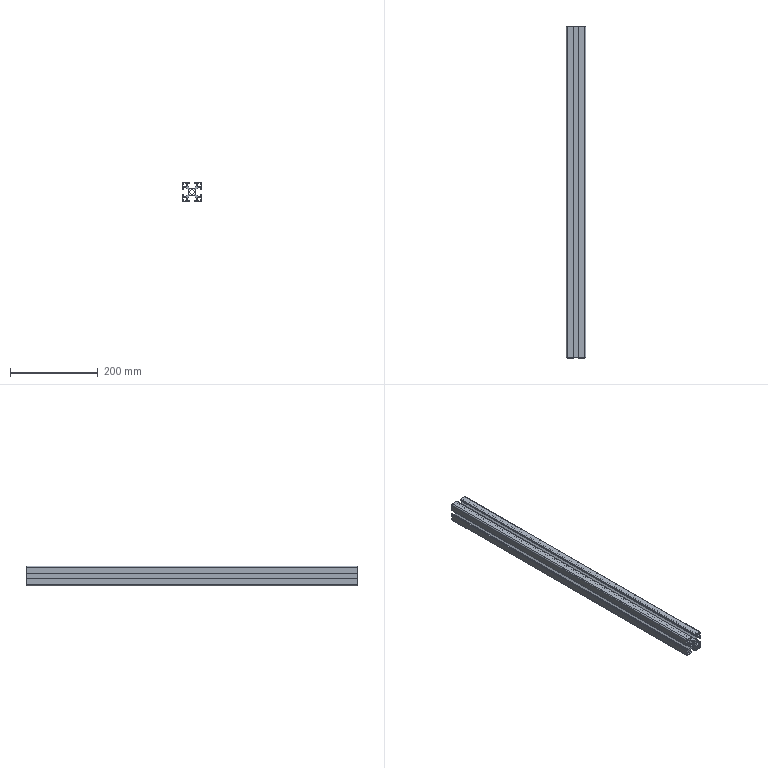Part | STEP file | 1 solid | 135 faces | box 45 x 757.5 x 45 mm | volume 524410 mm3 | plane 118 | cylinder 17 | commonest cylinder face diameters 10 x9 3 x4 5 x4